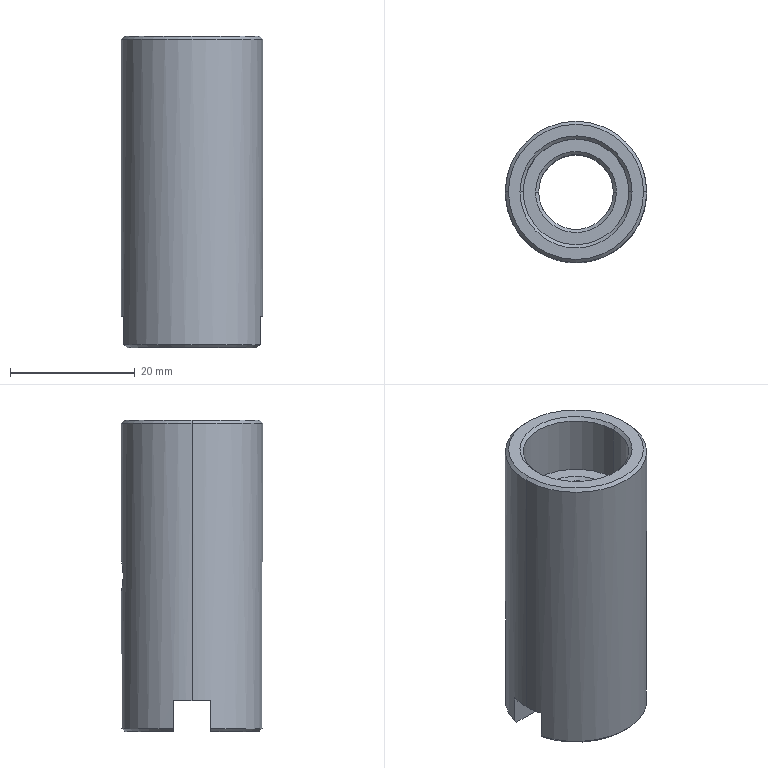Part | STEP file | 101000008215 | 1 solid | 28 faces | box 22.7 x 22.7 x 50 mm | volume 12976 mm3 | cone 10 | plane 10 | cylinder 8 | commonest cylinder face diameters 5 x2 12 x2 17 x2 22.7 x2
STEP:
#1=CARTESIAN_POINT('',(10.85,0.,50.));
#2=VERTEX_POINT('',#1);
#3=CARTESIAN_POINT('',(-10.85,0.,50.));
#4=VERTEX_POINT('',#3);
#5=CARTESIAN_POINT('',(0.,0.,50.));
#6=DIRECTION('',(0.,0.,-1.));
#7=AXIS2_PLACEMENT_3D('',#5,#6,$);
#8=CIRCLE('',#7,10.85);
#9=EDGE_CURVE('',#2,#4,#8,.F.);
#10=ORIENTED_EDGE('',*,*,#9,.F.);
#11=CARTESIAN_POINT('',(11.35,0.,49.5));
#12=VERTEX_POINT('',#11);
#13=CARTESIAN_POINT('',(353558.816,0.,-353497.966));
#14=DIRECTION('',(0.7071,0.,-0.7071));
#15=VECTOR('',#14,1.);
#16=LINE('',#13,#15);
#17=EDGE_CURVE('',#2,#12,#16,.T.);
#18=ORIENTED_EDGE('',*,*,#17,.T.);
#19=CARTESIAN_POINT('',(-11.35,0.,49.5));
#20=VERTEX_POINT('',#19);
#21=CARTESIAN_POINT('',(0.,0.,49.5));
#22=DIRECTION('',(0.,0.,-1.));
#23=AXIS2_PLACEMENT_3D('',#21,#22,$);
#24=CIRCLE('',#23,11.35);
#25=EDGE_CURVE('',#20,#12,#24,.T.);
#26=ORIENTED_EDGE('',*,*,#25,.F.);
#27=CARTESIAN_POINT('',(-353558.816,0.,-353497.966));
#28=DIRECTION('',(-0.7071,0.,-0.7071));
#29=VECTOR('',#28,1.);
#30=LINE('',#27,#29);
#31=EDGE_CURVE('',#4,#20,#30,.T.);
#32=ORIENTED_EDGE('',*,*,#31,.F.);
#33=EDGE_LOOP('',(#10,#18,#26,#32));
#34=FACE_OUTER_BOUND('',#33,.T.);
#35=CARTESIAN_POINT('',(0.,0.,50.));
#36=DIRECTION('',(0.,0.,-1.));
#37=DIRECTION('',(-1.,0.,0.));
#38=AXIS2_PLACEMENT_3D('',#35,#36,#37);
#39=CONICAL_SURFACE('',#38,10.85,0.7854);
#40=ADVANCED_FACE('',(#34),#39,.T.);
#41=CARTESIAN_POINT('',(0.,0.,50.));
#42=DIRECTION('',(0.,0.,1.));
#43=AXIS2_PLACEMENT_3D('',#41,#42,$);
#44=CIRCLE('',#43,10.85);
#45=EDGE_CURVE('',#4,#2,#44,.T.);
#46=ORIENTED_EDGE('',*,*,#45,.T.);
#47=ORIENTED_EDGE('',*,*,#9,.T.);
#48=EDGE_LOOP('',(#46,#47));
#49=FACE_OUTER_BOUND('',#48,.T.);
#50=CARTESIAN_POINT('',(9.,0.,50.));
#51=VERTEX_POINT('',#50);
#52=CARTESIAN_POINT('',(-9.,0.,50.));
#53=VERTEX_POINT('',#52);
#54=CARTESIAN_POINT('',(9.,0.,50.));
#55=CARTESIAN_POINT('',(9.,-0.8818,50.));
#56=CARTESIAN_POINT('',(8.892,-1.764,50.));
#57=CARTESIAN_POINT('',(8.676,-2.628,50.));
#58=CARTESIAN_POINT('',(8.037,-4.286,50.));
#59=CARTESIAN_POINT('',(7.016,-5.74,50.));
#60=CARTESIAN_POINT('',(6.419,-6.401,50.));
#61=CARTESIAN_POINT('',(5.075,-7.563,50.));
#62=CARTESIAN_POINT('',(3.49,-8.366,50.));
#63=CARTESIAN_POINT('',(2.652,-8.669,50.));
#64=CARTESIAN_POINT('',(0.9193,-9.061,50.));
#65=CARTESIAN_POINT('',(-0.8571,-9.025,50.));
#66=CARTESIAN_POINT('',(-1.739,-8.897,50.));
#67=CARTESIAN_POINT('',(-3.453,-8.428,50.));
#68=CARTESIAN_POINT('',(-5.003,-7.56,50.));
#69=CARTESIAN_POINT('',(-5.721,-7.032,50.));
#70=CARTESIAN_POINT('',(-7.012,-5.812,50.));
#71=CARTESIAN_POINT('',(-7.971,-4.317,50.));
#72=CARTESIAN_POINT('',(-8.357,-3.513,50.));
#73=CARTESIAN_POINT('',(-8.756,-2.324,50.));
#74=CARTESIAN_POINT('',(-8.945,-1.091,50.));
#75=CARTESIAN_POINT('',(-8.982,-0.7273,50.));
#76=CARTESIAN_POINT('',(-9.,-0.3637,50.));
#77=CARTESIAN_POINT('',(-9.,0.,50.));
#78=B_SPLINE_CURVE_WITH_KNOTS('',5,(#54,#55,#56,#57,#58,#59,#60,#61,#62,#63,#64,#65,#66,#67,#68,#69,#70,#71,#72,#73,#74,#75,#76,#77),.UNSPECIFIED.,.F.,.U.,(6,3,3,3,3,3,3,6),(0.,6.235,12.471,18.706,24.941,31.177,37.412,39.983),.UNSPECIFIED.);
#79=EDGE_CURVE('',#51,#53,#78,.T.);
#80=ORIENTED_EDGE('',*,*,#79,.T.);
#81=CARTESIAN_POINT('',(-9.,0.,50.));
#82=CARTESIAN_POINT('',(-9.,0.8818,50.));
#83=CARTESIAN_POINT('',(-8.892,1.764,50.));
#84=CARTESIAN_POINT('',(-8.676,2.628,50.));
#85=CARTESIAN_POINT('',(-8.037,4.286,50.));
#86=CARTESIAN_POINT('',(-7.016,5.74,50.));
#87=CARTESIAN_POINT('',(-6.419,6.401,50.));
#88=CARTESIAN_POINT('',(-5.075,7.563,50.));
#89=CARTESIAN_POINT('',(-3.49,8.366,50.));
#90=CARTESIAN_POINT('',(-2.652,8.669,50.));
#91=CARTESIAN_POINT('',(-0.9193,9.061,50.));
#92=CARTESIAN_POINT('',(0.8571,9.025,50.));
#93=CARTESIAN_POINT('',(1.739,8.897,50.));
#94=CARTESIAN_POINT('',(3.453,8.428,50.));
#95=CARTESIAN_POINT('',(5.003,7.56,50.));
#96=CARTESIAN_POINT('',(5.721,7.032,50.));
#97=CARTESIAN_POINT('',(7.012,5.812,50.));
#98=CARTESIAN_POINT('',(7.971,4.317,50.));
#99=CARTESIAN_POINT('',(8.357,3.513,50.));
#100=CARTESIAN_POINT('',(8.756,2.324,50.));
#101=CARTESIAN_POINT('',(8.945,1.091,50.));
#102=CARTESIAN_POINT('',(8.982,0.7273,50.));
#103=CARTESIAN_POINT('',(9.,0.3637,50.));
#104=CARTESIAN_POINT('',(9.,0.,50.));
#105=B_SPLINE_CURVE_WITH_KNOTS('',5,(#81,#82,#83,#84,#85,#86,#87,#88,#89,#90,#91,#92,#93,#94,#95,#96,#97,#98,#99,#100,#101,#102,#103,#104),.UNSPECIFIED.,.F.,.U.,(6,3,3,3,3,3,3,6),(0.,6.235,12.471,18.706,24.941,31.177,37.412,39.983),.UNSPECIFIED.);
#106=EDGE_CURVE('',#53,#51,#105,.T.);
#107=ORIENTED_EDGE('',*,*,#106,.T.);
#108=EDGE_LOOP('',(#80,#107));
#109=FACE_BOUND('',#108,.T.);
#110=CARTESIAN_POINT('',(0.,0.,50.));
#111=DIRECTION('',(0.,0.,1.));
#112=DIRECTION('',(1.,0.,0.));
#113=AXIS2_PLACEMENT_3D('',#110,#111,#112);
#114=PLANE('',#113);
#115=ADVANCED_FACE('',(#49,#109),#114,.T.);
#116=ORIENTED_EDGE('',*,*,#17,.F.);
#117=ORIENTED_EDGE('',*,*,#45,.F.);
#118=ORIENTED_EDGE('',*,*,#31,.T.);
#119=CARTESIAN_POINT('',(0.,0.,49.5));
#120=DIRECTION('',(0.,0.,-1.));
#121=AXIS2_PLACEMENT_3D('',#119,#120,$);
#122=CIRCLE('',#121,11.35);
#123=EDGE_CURVE('',#12,#20,#122,.T.);
#124=ORIENTED_EDGE('',*,*,#123,.F.);
#125=EDGE_LOOP('',(#116,#117,#118,#124));
#126=FACE_OUTER_BOUND('',#125,.T.);
#127=CARTESIAN_POINT('',(0.,0.,50.));
#128=DIRECTION('',(0.,0.,-1.));
#129=DIRECTION('',(1.,0.,0.));
#130=AXIS2_PLACEMENT_3D('',#127,#128,#129);
#131=CONICAL_SURFACE('',#130,10.85,0.7854);
#132=ADVANCED_FACE('',(#126),#131,.T.);
#133=ORIENTED_EDGE('',*,*,#25,.T.);
#134=CARTESIAN_POINT('',(11.35,0.,5.));
#135=VERTEX_POINT('',#134);
#136=CARTESIAN_POINT('',(11.35,0.,50.));
#137=DIRECTION('',(0.,0.,-1.));
#138=VECTOR('',#137,1.);
#139=LINE('',#136,#138);
#140=EDGE_CURVE('',#12,#135,#139,.T.);
#141=ORIENTED_EDGE('',*,*,#140,.T.);
#142=CARTESIAN_POINT('',(10.946,3.,5.));
#143=VERTEX_POINT('',#142);
#144=CARTESIAN_POINT('',(0.,0.,5.));
#145=DIRECTION('',(0.,0.,-1.));
#146=AXIS2_PLACEMENT_3D('',#144,#145,$);
#147=CIRCLE('',#146,11.35);
#148=EDGE_CURVE('',#135,#143,#147,.F.);
#149=ORIENTED_EDGE('',*,*,#148,.T.);
#150=CARTESIAN_POINT('',(10.946,3.,0.5));
#151=VERTEX_POINT('',#150);
#152=CARTESIAN_POINT('',(10.946,3.,50.));
#153=DIRECTION('',(0.,0.,-1.));
#154=VECTOR('',#153,1.);
#155=LINE('',#152,#154);
#156=EDGE_CURVE('',#143,#151,#155,.T.);
#157=ORIENTED_EDGE('',*,*,#156,.T.);
#158=CARTESIAN_POINT('',(-10.946,3.,0.5));
#159=VERTEX_POINT('',#158);
#160=CARTESIAN_POINT('',(0.,0.,0.5));
#161=DIRECTION('',(0.,0.,-1.));
#162=AXIS2_PLACEMENT_3D('',#160,#161,$);
#163=CIRCLE('',#162,11.35);
#164=EDGE_CURVE('',#151,#159,#163,.F.);
#165=ORIENTED_EDGE('',*,*,#164,.T.);
#166=CARTESIAN_POINT('',(-10.946,3.,5.));
#167=VERTEX_POINT('',#166);
#168=CARTESIAN_POINT('',(-10.946,3.,50.));
#169=DIRECTION('',(0.,0.,-1.));
#170=VECTOR('',#169,1.);
#171=LINE('',#168,#170);
#172=EDGE_CURVE('',#159,#167,#171,.F.);
#173=ORIENTED_EDGE('',*,*,#172,.T.);
#174=CARTESIAN_POINT('',(-11.35,0.,5.));
#175=VERTEX_POINT('',#174);
#176=CARTESIAN_POINT('',(0.,0.,5.));
#177=DIRECTION('',(0.,0.,-1.));
#178=AXIS2_PLACEMENT_3D('',#176,#177,$);
#179=CIRCLE('',#178,11.35);
#180=EDGE_CURVE('',#167,#175,#179,.F.);
#181=ORIENTED_EDGE('',*,*,#180,.T.);
#182=CARTESIAN_POINT('',(-11.35,0.,50.));
#183=DIRECTION('',(0.,0.,-1.));
#184=VECTOR('',#183,1.);
#185=LINE('',#182,#184);
#186=EDGE_CURVE('',#20,#175,#185,.T.);
#187=ORIENTED_EDGE('',*,*,#186,.F.);
#188=EDGE_LOOP('',(#133,#141,#149,#157,#165,#173,#181,#187));
#189=FACE_OUTER_BOUND('',#188,.T.);
#190=CARTESIAN_POINT('',(0.,11.35,27.5));
#191=VERTEX_POINT('',#190);
#192=CARTESIAN_POINT('',(0.,11.35,22.5));
#193=VERTEX_POINT('',#192);
#194=CARTESIAN_POINT('',(0.,11.35,27.5));
#195=CARTESIAN_POINT('',(-0.2311,11.35,27.5));
#196=CARTESIAN_POINT('',(-0.4593,11.344,27.474));
#197=CARTESIAN_POINT('',(-0.687,11.332,27.42));
#198=CARTESIAN_POINT('',(-1.051,11.305,27.289));
#199=CARTESIAN_POINT('',(-1.38,11.267,27.093));
#200=CARTESIAN_POINT('',(-1.506,11.251,27.004));
#201=CARTESIAN_POINT('',(-1.922,11.191,26.66));
#202=CARTESIAN_POINT('',(-2.236,11.13,26.214));
#203=CARTESIAN_POINT('',(-2.398,11.094,25.852));
#204=CARTESIAN_POINT('',(-2.52,11.067,25.32));
#205=CARTESIAN_POINT('',(-2.497,11.072,24.78));
#206=CARTESIAN_POINT('',(-2.479,11.076,24.626));
#207=CARTESIAN_POINT('',(-2.404,11.093,24.249));
#208=CARTESIAN_POINT('',(-2.259,11.124,23.893));
#209=CARTESIAN_POINT('',(-2.148,11.146,23.689));
#210=CARTESIAN_POINT('',(-1.878,11.196,23.31));
#211=CARTESIAN_POINT('',(-1.531,11.248,23.003));
#212=CARTESIAN_POINT('',(-1.339,11.273,22.87));
#213=CARTESIAN_POINT('',(-0.9666,11.313,22.671));
#214=CARTESIAN_POINT('',(-0.5631,11.338,22.553));
#215=CARTESIAN_POINT('',(-0.3767,11.346,22.518));
#216=CARTESIAN_POINT('',(-0.1878,11.35,22.5));
#217=CARTESIAN_POINT('',(0.,11.35,22.5));
#218=B_SPLINE_CURVE_WITH_KNOTS('',5,(#194,#195,#196,#197,#198,#199,#200,#201,#202,#203,#204,#205,#206,#207,#208,#209,#210,#211,#212,#213,#214,#215,#216,#217),.UNSPECIFIED.,.F.,.U.,(6,3,3,3,3,3,3,6),(0.,1.627,2.724,5.45,6.533,8.168,9.815,11.146),.UNSPECIFIED.);
#219=EDGE_CURVE('',#191,#193,#218,.T.);
#220=ORIENTED_EDGE('',*,*,#219,.T.);
#221=CARTESIAN_POINT('',(0.,11.35,22.5));
#222=CARTESIAN_POINT('',(0.2297,11.35,22.5));
#223=CARTESIAN_POINT('',(0.4594,11.344,22.527));
#224=CARTESIAN_POINT('',(0.6875,11.332,22.58));
#225=CARTESIAN_POINT('',(1.051,11.305,22.711));
#226=CARTESIAN_POINT('',(1.381,11.267,22.908));
#227=CARTESIAN_POINT('',(1.508,11.25,22.997));
#228=CARTESIAN_POINT('',(1.745,11.216,23.193));
#229=CARTESIAN_POINT('',(1.95,11.182,23.425));
#230=CARTESIAN_POINT('',(2.044,11.165,23.549));
#231=CARTESIAN_POINT('',(2.252,11.125,23.871));
#232=CARTESIAN_POINT('',(2.395,11.095,24.229));
#233=CARTESIAN_POINT('',(2.455,11.081,24.455));
#234=CARTESIAN_POINT('',(2.513,11.068,24.835));
#235=CARTESIAN_POINT('',(2.498,11.072,25.218));
#236=CARTESIAN_POINT('',(2.479,11.076,25.371));
#237=CARTESIAN_POINT('',(2.42,11.089,25.673));
#238=CARTESIAN_POINT('',(2.315,11.112,25.962));
#239=CARTESIAN_POINT('',(2.252,11.125,26.101));
#240=CARTESIAN_POINT('',(2.104,11.154,26.373));
#241=CARTESIAN_POINT('',(1.915,11.188,26.618));
#242=CARTESIAN_POINT('',(1.811,11.205,26.734));
#243=CARTESIAN_POINT('',(1.451,11.261,27.076));
#244=CARTESIAN_POINT('',(1.014,11.311,27.323));
#245=CARTESIAN_POINT('',(0.6857,11.337,27.441));
#246=CARTESIAN_POINT('',(0.3439,11.35,27.5));
#247=CARTESIAN_POINT('',(0.,11.35,27.5));
#248=B_SPLINE_CURVE_WITH_KNOTS('',5,(#221,#222,#223,#224,#225,#226,#227,#228,#229,#230,#231,#232,#233,#234,#235,#236,#237,#238,#239,#240,#241,#242,#243,#244,#245,#246,#247),.UNSPECIFIED.,.F.,.U.,(6,3,3,3,3,3,3,3,6),(0.,1.629,2.725,3.823,5.451,6.53,7.624,8.727,11.154),.UNSPECIFIED.);
#249=EDGE_CURVE('',#193,#191,#248,.T.);
#250=ORIENTED_EDGE('',*,*,#249,.T.);
#251=EDGE_LOOP('',(#220,#250));
#252=FACE_BOUND('',#251,.T.);
#253=CARTESIAN_POINT('',(0.,0.,50.));
#254=DIRECTION('',(0.,0.,-1.));
#255=DIRECTION('',(-1.,0.,0.));
#256=AXIS2_PLACEMENT_3D('',#253,#254,#255);
#257=CYLINDRICAL_SURFACE('',#256,11.35);
#258=ADVANCED_FACE('',(#189,#252),#257,.T.);
#259=CARTESIAN_POINT('',(-8.5,0.,49.5));
#260=VERTEX_POINT('',#259);
#261=CARTESIAN_POINT('',(8.5,0.,49.5));
#262=VERTEX_POINT('',#261);
#263=CARTESIAN_POINT('',(0.,0.,49.5));
#264=DIRECTION('',(0.,0.,1.));
#265=AXIS2_PLACEMENT_3D('',#263,#264,$);
#266=CIRCLE('',#265,8.5);
#267=EDGE_CURVE('',#260,#262,#266,.T.);
#268=ORIENTED_EDGE('',*,*,#267,.F.);
#269=CARTESIAN_POINT('',(-353557.641,0.,353598.641));
#270=DIRECTION('',(-0.7071,0.,0.7071));
#271=VECTOR('',#270,1.);
#272=LINE('',#269,#271);
#273=EDGE_CURVE('',#260,#53,#272,.T.);
#274=ORIENTED_EDGE('',*,*,#273,.T.);
#275=ORIENTED_EDGE('',*,*,#79,.F.);
#276=CARTESIAN_POINT('',(353557.641,0.,353598.641));
#277=DIRECTION('',(0.7071,0.,0.7071));
#278=VECTOR('',#277,1.);
#279=LINE('',#276,#278);
#280=EDGE_CURVE('',#262,#51,#279,.T.);
#281=ORIENTED_EDGE('',*,*,#280,.F.);
#282=EDGE_LOOP('',(#268,#274,#275,#281));
#283=FACE_OUTER_BOUND('',#282,.T.);
#284=CARTESIAN_POINT('',(0.,0.,49.5));
#285=DIRECTION('',(0.,0.,1.));
#286=DIRECTION('',(-1.,0.,0.));
#287=AXIS2_PLACEMENT_3D('',#284,#285,#286);
#288=CONICAL_SURFACE('',#287,8.5,0.7854);
#289=ADVANCED_FACE('',(#283),#288,.F.);
#290=ORIENTED_EDGE('',*,*,#273,.F.);
#291=CARTESIAN_POINT('',(0.,0.,49.5));
#292=DIRECTION('',(0.,0.,1.));
#293=AXIS2_PLACEMENT_3D('',#291,#292,$);
#294=CIRCLE('',#293,8.5);
#295=EDGE_CURVE('',#262,#260,#294,.T.);
#296=ORIENTED_EDGE('',*,*,#295,.F.);
#297=ORIENTED_EDGE('',*,*,#280,.T.);
#298=ORIENTED_EDGE('',*,*,#106,.F.);
#299=EDGE_LOOP('',(#290,#296,#297,#298));
#300=FACE_OUTER_BOUND('',#299,.T.);
#301=CARTESIAN_POINT('',(0.,0.,49.5));
#302=DIRECTION('',(0.,0.,1.));
#303=DIRECTION('',(1.,0.,0.));
#304=AXIS2_PLACEMENT_3D('',#301,#302,#303);
#305=CONICAL_SURFACE('',#304,8.5,0.7854);
#306=ADVANCED_FACE('',(#300),#305,.F.);
#307=ORIENTED_EDGE('',*,*,#140,.F.);
#308=ORIENTED_EDGE('',*,*,#123,.T.);
#309=ORIENTED_EDGE('',*,*,#186,.T.);
#310=CARTESIAN_POINT('',(-10.946,-3.,5.));
#311=VERTEX_POINT('',#310);
#312=CARTESIAN_POINT('',(0.,0.,5.));
#313=DIRECTION('',(0.,0.,-1.));
#314=AXIS2_PLACEMENT_3D('',#312,#313,$);
#315=CIRCLE('',#314,11.35);
#316=EDGE_CURVE('',#175,#311,#315,.F.);
#317=ORIENTED_EDGE('',*,*,#316,.T.);
#318=CARTESIAN_POINT('',(-10.946,-3.,0.5));
#319=VERTEX_POINT('',#318);
#320=CARTESIAN_POINT('',(-10.946,-3.,50.));
#321=DIRECTION('',(0.,0.,-1.));
#322=VECTOR('',#321,1.);
#323=LINE('',#320,#322);
#324=EDGE_CURVE('',#311,#319,#323,.T.);
#325=ORIENTED_EDGE('',*,*,#324,.T.);
#326=CARTESIAN_POINT('',(10.946,-3.,0.5));
#327=VERTEX_POINT('',#326);
#328=CARTESIAN_POINT('',(0.,0.,0.5));
#329=DIRECTION('',(0.,0.,-1.));
#330=AXIS2_PLACEMENT_3D('',#328,#329,$);
#331=CIRCLE('',#330,11.35);
#332=EDGE_CURVE('',#319,#327,#331,.F.);
#333=ORIENTED_EDGE('',*,*,#332,.T.);
#334=CARTESIAN_POINT('',(10.946,-3.,5.));
#335=VERTEX_POINT('',#334);
#336=CARTESIAN_POINT('',(10.946,-3.,50.));
#337=DIRECTION('',(0.,0.,-1.));
#338=VECTOR('',#337,1.);
#339=LINE('',#336,#338);
#340=EDGE_CURVE('',#327,#335,#339,.F.);
#341=ORIENTED_EDGE('',*,*,#340,.T.);
#342=CARTESIAN_POINT('',(0.,0.,5.));
#343=DIRECTION('',(0.,0.,-1.));
#344=AXIS2_PLACEMENT_3D('',#342,#343,$);
#345=CIRCLE('',#344,11.35);
#346=EDGE_CURVE('',#335,#135,#345,.F.);
#347=ORIENTED_EDGE('',*,*,#346,.T.);
#348=EDGE_LOOP('',(#307,#308,#309,#317,#325,#333,#341,#347));
#349=FACE_OUTER_BOUND('',#348,.T.);
#350=CARTESIAN_POINT('',(0.,0.,50.));
#351=DIRECTION('',(0.,0.,-1.));
#352=DIRECTION('',(1.,0.,0.));
#353=AXIS2_PLACEMENT_3D('',#350,#351,#352);
#354=CYLINDRICAL_SURFACE('',#353,11.35);
#355=ADVANCED_FACE('',(#349),#354,.T.);
#356=CARTESIAN_POINT('',(5.196,-3.,5.));
#357=VERTEX_POINT('',#356);
#358=CARTESIAN_POINT('',(6.,0.,5.));
#359=VERTEX_POINT('',#358);
#360=CARTESIAN_POINT('',(0.00000002,-0.000000005,5.));
#361=DIRECTION('',(0.,0.,1.));
#362=AXIS2_PLACEMENT_3D('',#360,#361,$);
#363=CIRCLE('',#362,6.);
#364=EDGE_CURVE('',#357,#359,#363,.T.);
#365=ORIENTED_EDGE('',*,*,#364,.T.);
#366=CARTESIAN_POINT('',(5.196,3.,5.));
#367=VERTEX_POINT('',#366);
#368=CARTESIAN_POINT('',(0.00000002,0.000000005,5.));
#369=DIRECTION('',(0.,0.,1.));
#370=AXIS2_PLACEMENT_3D('',#368,#369,$);
#371=CIRCLE('',#370,6.);
#372=EDGE_CURVE('',#359,#367,#371,.T.);
#373=ORIENTED_EDGE('',*,*,#372,.T.);
#374=CARTESIAN_POINT('',(8.071,3.,5.));
#375=DIRECTION('',(1.,0.,0.));
#376=VECTOR('',#375,1.);
#377=LINE('',#374,#376);
#378=EDGE_CURVE('',#367,#143,#377,.T.);
#379=ORIENTED_EDGE('',*,*,#378,.T.);
#380=ORIENTED_EDGE('',*,*,#148,.F.);
#381=ORIENTED_EDGE('',*,*,#346,.F.);
#382=CARTESIAN_POINT('',(8.071,-3.,5.));
#383=DIRECTION('',(1.,0.,0.));
#384=VECTOR('',#383,1.);
#385=LINE('',#382,#384);
#386=EDGE_CURVE('',#357,#335,#385,.T.);
#387=ORIENTED_EDGE('',*,*,#386,.F.);
#388=EDGE_LOOP('',(#365,#373,#379,#380,#381,#387));
#389=FACE_OUTER_BOUND('',#388,.T.);
#390=CARTESIAN_POINT('',(-11.35,3.,5.));
#391=DIRECTION('',(0.,0.,1.));
#392=DIRECTION('',(1.,0.,0.));
#393=AXIS2_PLACEMENT_3D('',#390,#391,#392);
#394=PLANE('',#393);
#395=ADVANCED_FACE('',(#389),#394,.F.);
#396=CARTESIAN_POINT('',(5.766,3.,0.));
#397=VERTEX_POINT('',#396);
#398=CARTESIAN_POINT('',(10.427,3.,0.));
#399=VERTEX_POINT('',#398);
#400=CARTESIAN_POINT('',(8.097,3.,0.));
#401=DIRECTION('',(1.,0.,0.));
#402=VECTOR('',#401,1.);
#403=LINE('',#400,#402);
#404=EDGE_CURVE('',#397,#399,#403,.T.);
#405=ORIENTED_EDGE('',*,*,#404,.T.);
#406=CARTESIAN_POINT('',(10.427,3.,0.));
#407=CARTESIAN_POINT('',(10.531,3.,0.09991));
#408=CARTESIAN_POINT('',(10.635,3.,0.1999));
#409=CARTESIAN_POINT('',(10.739,3.,0.2999));
#410=CARTESIAN_POINT('',(10.843,3.,0.3999));
#411=CARTESIAN_POINT('',(10.946,3.,0.5));
#412=B_SPLINE_CURVE_WITH_KNOTS('',5,(#406,#407,#408,#409,#410,#411),.UNSPECIFIED.,.F.,.U.,(6,6),(0.,1.02),.UNSPECIFIED.);
#413=EDGE_CURVE('',#399,#151,#412,.T.);
#414=ORIENTED_EDGE('',*,*,#413,.T.);
#415=ORIENTED_EDGE('',*,*,#156,.F.);
#416=ORIENTED_EDGE('',*,*,#378,.F.);
#417=CARTESIAN_POINT('',(5.196,3.,0.5));
#418=VERTEX_POINT('',#417);
#419=CARTESIAN_POINT('',(5.196,3.,2.75));
#420=DIRECTION('',(0.,0.,-1.));
#421=VECTOR('',#420,1.);
#422=LINE('',#419,#421);
#423=EDGE_CURVE('',#367,#418,#422,.T.);
#424=ORIENTED_EDGE('',*,*,#423,.T.);
#425=CARTESIAN_POINT('',(5.196,3.,0.5));
#426=CARTESIAN_POINT('',(5.311,3.,0.4007));
#427=CARTESIAN_POINT('',(5.425,3.,0.301));
#428=CARTESIAN_POINT('',(5.539,3.,0.201));
#429=CARTESIAN_POINT('',(5.653,3.,0.1006));
#430=CARTESIAN_POINT('',(5.766,3.,0.));
#431=B_SPLINE_CURVE_WITH_KNOTS('',5,(#425,#426,#427,#428,#429,#430),.UNSPECIFIED.,.F.,.U.,(6,6),(0.,1.072),.UNSPECIFIED.);
#432=EDGE_CURVE('',#418,#397,#431,.T.);
#433=ORIENTED_EDGE('',*,*,#432,.T.);
#434=EDGE_LOOP('',(#405,#414,#415,#416,#424,#433));
#435=FACE_OUTER_BOUND('',#434,.T.);
#436=CARTESIAN_POINT('',(-11.35,3.,5.));
#437=DIRECTION('',(0.,1.,0.));
#438=DIRECTION('',(0.,0.,1.));
#439=AXIS2_PLACEMENT_3D('',#436,#437,#438);
#440=PLANE('',#439);
#441=ADVANCED_FACE('',(#435),#440,.F.);
#442=ORIENTED_EDGE('',*,*,#413,.F.);
#443=CARTESIAN_POINT('',(-10.427,3.,0.));
#444=VERTEX_POINT('',#443);
#445=CARTESIAN_POINT('',(0.,0.,0.));
#446=DIRECTION('',(0.,0.,1.));
#447=AXIS2_PLACEMENT_3D('',#445,#446,$);
#448=CIRCLE('',#447,10.85);
#449=EDGE_CURVE('',#444,#399,#448,.F.);
#450=ORIENTED_EDGE('',*,*,#449,.F.);
#451=CARTESIAN_POINT('',(-10.946,3.,0.5));
#452=CARTESIAN_POINT('',(-10.769,3.,0.3286));
#453=CARTESIAN_POINT('',(-10.595,3.,0.1619));
#454=CARTESIAN_POINT('',(-10.427,3.,0.));
#455=B_SPLINE_CURVE_WITH_KNOTS('',3,(#451,#452,#453,#454),.UNSPECIFIED.,.F.,.U.,(4,4),(0.,1.619),.UNSPECIFIED.);
#456=EDGE_CURVE('',#159,#444,#455,.T.);
#457=ORIENTED_EDGE('',*,*,#456,.F.);
#458=ORIENTED_EDGE('',*,*,#164,.F.);
#459=EDGE_LOOP('',(#442,#450,#457,#458));
#460=FACE_OUTER_BOUND('',#459,.T.);
#461=CARTESIAN_POINT('',(0.,0.,0.5));
#462=DIRECTION('',(0.,0.,1.));
#463=DIRECTION('',(1.,0.,0.));
#464=AXIS2_PLACEMENT_3D('',#461,#462,#463);
#465=CONICAL_SURFACE('',#464,11.35,0.7854);
#466=ADVANCED_FACE('',(#460),#465,.T.);
#467=ORIENTED_EDGE('',*,*,#172,.F.);
#468=ORIENTED_EDGE('',*,*,#456,.T.);
#469=CARTESIAN_POINT('',(-5.766,3.,0.));
#470=VERTEX_POINT('',#469);
#471=CARTESIAN_POINT('',(-8.097,3.,0.));
#472=DIRECTION('',(1.,0.,0.));
#473=VECTOR('',#472,1.);
#474=LINE('',#471,#473);
#475=EDGE_CURVE('',#444,#470,#474,.T.);
#476=ORIENTED_EDGE('',*,*,#475,.T.);
#477=CARTESIAN_POINT('',(-5.196,3.,0.5));
#478=VERTEX_POINT('',#477);
#479=CARTESIAN_POINT('',(-5.766,3.,0.));
#480=CARTESIAN_POINT('',(-5.653,3.,0.1006));
#481=CARTESIAN_POINT('',(-5.539,3.,0.201));
#482=CARTESIAN_POINT('',(-5.425,3.,0.301));
#483=CARTESIAN_POINT('',(-5.311,3.,0.4007));
#484=CARTESIAN_POINT('',(-5.196,3.,0.5));
#485=B_SPLINE_CURVE_WITH_KNOTS('',5,(#479,#480,#481,#482,#483,#484),.UNSPECIFIED.,.F.,.U.,(6,6),(0.,1.072),.UNSPECIFIED.);
#486=EDGE_CURVE('',#470,#478,#485,.T.);
#487=ORIENTED_EDGE('',*,*,#486,.T.);
#488=CARTESIAN_POINT('',(-5.196,3.,5.));
#489=VERTEX_POINT('',#488);
#490=CARTESIAN_POINT('',(-5.196,3.,2.75));
#491=DIRECTION('',(0.,0.,1.));
#492=VECTOR('',#491,1.);
#493=LINE('',#490,#492);
#494=EDGE_CURVE('',#478,#489,#493,.T.);
#495=ORIENTED_EDGE('',*,*,#494,.T.);
#496=CARTESIAN_POINT('',(-8.071,3.,5.));
#497=DIRECTION('',(1.,0.,0.));
#498=VECTOR('',#497,1.);
#499=LINE('',#496,#498);
#500=EDGE_CURVE('',#167,#489,#499,.T.);
#501=ORIENTED_EDGE('',*,*,#500,.F.);
#502=EDGE_LOOP('',(#467,#468,#476,#487,#495,#501));
#503=FACE_OUTER_BOUND('',#502,.T.);
#504=CARTESIAN_POINT('',(-11.35,3.,5.));
#505=DIRECTION('',(0.,1.,0.));
#506=DIRECTION('',(0.,0.,1.));
#507=AXIS2_PLACEMENT_3D('',#504,#505,#506);
#508=PLANE('',#507);
#509=ADVANCED_FACE('',(#503),#508,.F.);
#510=CARTESIAN_POINT('',(-6.,0.,5.));
#511=VERTEX_POINT('',#510);
#512=CARTESIAN_POINT('',(-0.000000021,0.000000005,5.));
#513=DIRECTION('',(0.,0.,1.));
#514=AXIS2_PLACEMENT_3D('',#512,#513,$);
#515=CIRCLE('',#514,6.);
#516=EDGE_CURVE('',#489,#511,#515,.T.);
#517=ORIENTED_EDGE('',*,*,#516,.T.);
#518=CARTESIAN_POINT('',(-5.196,-3.,5.));
#519=VERTEX_POINT('',#518);
#520=CARTESIAN_POINT('',(-0.000000021,-0.000000005,5.));
#521=DIRECTION('',(0.,0.,1.));
#522=AXIS2_PLACEMENT_3D('',#520,#521,$);
#523=CIRCLE('',#522,6.);
#524=EDGE_CURVE('',#511,#519,#523,.T.);
#525=ORIENTED_EDGE('',*,*,#524,.T.);
#526=CARTESIAN_POINT('',(-8.071,-3.,5.));
#527=DIRECTION('',(1.,0.,0.));
#528=VECTOR('',#527,1.);
#529=LINE('',#526,#528);
#530=EDGE_CURVE('',#311,#519,#529,.T.);
#531=ORIENTED_EDGE('',*,*,#530,.F.);
#532=ORIENTED_EDGE('',*,*,#316,.F.);
#533=ORIENTED_EDGE('',*,*,#180,.F.);
#534=ORIENTED_EDGE('',*,*,#500,.T.);
#535=EDGE_LOOP('',(#517,#525,#531,#532,#533,#534));
#536=FACE_OUTER_BOUND('',#535,.T.);
#537=CARTESIAN_POINT('',(-11.35,3.,5.));
#538=DIRECTION('',(0.,0.,1.));
#539=DIRECTION('',(1.,0.,0.));
#540=AXIS2_PLACEMENT_3D('',#537,#538,#539);
#541=PLANE('',#540);
#542=ADVANCED_FACE('',(#536),#541,.F.);
#543=CARTESIAN_POINT('',(0.,6.,27.5));
#544=VERTEX_POINT('',#543);
#545=CARTESIAN_POINT('',(0.,6.,22.5));
#546=VERTEX_POINT('',#545);
#547=CARTESIAN_POINT('',(0.,6.,27.5));
#548=CARTESIAN_POINT('',(-0.3045,6.,27.5));
#549=CARTESIAN_POINT('',(-0.6041,5.981,27.454));
#550=CARTESIAN_POINT('',(-0.8951,5.943,27.363));
#551=CARTESIAN_POINT('',(-1.308,5.864,27.162));
#552=CARTESIAN_POINT('',(-1.663,5.767,26.877));
#553=CARTESIAN_POINT('',(-1.769,5.735,26.777));
#554=CARTESIAN_POINT('',(-1.976,5.667,26.55));
#555=CARTESIAN_POINT('',(-2.147,5.604,26.294));
#556=CARTESIAN_POINT('',(-2.222,5.574,26.16));
#557=CARTESIAN_POINT('',(-2.349,5.522,25.888));
#558=CARTESIAN_POINT('',(-2.434,5.484,25.599));
#559=CARTESIAN_POINT('',(-2.465,5.47,25.456));
#560=CARTESIAN_POINT('',(-2.506,5.452,25.162));
#561=CARTESIAN_POINT('',(-2.503,5.453,24.864));
#562=CARTESIAN_POINT('',(-2.49,5.459,24.713));
#563=CARTESIAN_POINT('',(-2.442,5.481,24.417));
#564=CARTESIAN_POINT('',(-2.352,5.52,24.133));
#565=CARTESIAN_POINT('',(-2.296,5.544,23.994));
#566=CARTESIAN_POINT('',(-2.161,5.599,23.721));
#567=CARTESIAN_POINT('',(-1.988,5.662,23.472));
#568=CARTESIAN_POINT('',(-1.89,5.696,23.353));
#569=CARTESIAN_POINT('',(-1.628,5.78,23.079));
#570=CARTESIAN_POINT('',(-1.318,5.858,22.858));
#571=CARTESIAN_POINT('',(-1.115,5.902,22.745));
#572=CARTESIAN_POINT('',(-0.7752,5.956,22.605));
#573=CARTESIAN_POINT('',(-0.415,5.988,22.529));
#574=CARTESIAN_POINT('',(-0.2773,5.996,22.51));
#575=CARTESIAN_POINT('',(-0.1387,6.,22.5));
#576=CARTESIAN_POINT('',(0.,6.,22.5));
#577=B_SPLINE_CURVE_WITH_KNOTS('',5,(#547,#548,#549,#550,#551,#552,#553,#554,#555,#556,#557,#558,#559,#560,#561,#562,#563,#564,#565,#566,#567,#568,#569,#570,#571,#572,#573,#574,#575,#576),.UNSPECIFIED.,.F.,.U.,(6,3,3,3,3,3,3,3,3,6),(0.,2.145,3.277,4.365,5.422,6.468,7.54,8.653,10.281,11.264),.UNSPECIFIED.);
#578=EDGE_CURVE('',#544,#546,#577,.T.);
#579=ORIENTED_EDGE('',*,*,#578,.T.);
#580=CARTESIAN_POINT('',(0.,11.5,22.5));
#581=DIRECTION('',(0.,1.,0.));
#582=VECTOR('',#581,1.);
#583=LINE('',#580,#582);
#584=EDGE_CURVE('',#546,#193,#583,.T.);
#585=ORIENTED_EDGE('',*,*,#584,.T.);
#586=ORIENTED_EDGE('',*,*,#219,.F.);
#587=CARTESIAN_POINT('',(0.,11.5,27.5));
#588=DIRECTION('',(0.,1.,0.));
#589=VECTOR('',#588,1.);
#590=LINE('',#587,#589);
#591=EDGE_CURVE('',#544,#191,#590,.T.);
#592=ORIENTED_EDGE('',*,*,#591,.F.);
#593=EDGE_LOOP('',(#579,#585,#586,#592));
#594=FACE_OUTER_BOUND('',#593,.T.);
#595=CARTESIAN_POINT('',(0.,11.5,25.));
#596=DIRECTION('',(0.,1.,0.));
#597=DIRECTION('',(0.,0.,-1.));
#598=AXIS2_PLACEMENT_3D('',#595,#596,#597);
#599=CYLINDRICAL_SURFACE('',#598,2.5);
#600=ADVANCED_FACE('',(#594),#599,.F.);
#601=ORIENTED_EDGE('',*,*,#584,.F.);
#602=CARTESIAN_POINT('',(0.,6.,22.5));
#603=CARTESIAN_POINT('',(0.3012,6.,22.5));
#604=CARTESIAN_POINT('',(0.6054,5.98,22.545));
#605=CARTESIAN_POINT('',(0.8939,5.943,22.636));
#606=CARTESIAN_POINT('',(1.308,5.864,22.838));
#607=CARTESIAN_POINT('',(1.661,5.768,23.121));
#608=CARTESIAN_POINT('',(1.765,5.736,23.22));
#609=CARTESIAN_POINT('',(1.973,5.669,23.445));
#610=CARTESIAN_POINT('',(2.144,5.605,23.701));
#611=CARTESIAN_POINT('',(2.22,5.575,23.835));
#612=CARTESIAN_POINT('',(2.378,5.51,24.172));
#613=CARTESIAN_POINT('',(2.471,5.468,24.535));
#614=CARTESIAN_POINT('',(2.503,5.452,24.759));
#615=CARTESIAN_POINT('',(2.521,5.445,25.369));
#616=CARTESIAN_POINT('',(2.356,5.521,25.959));
#617=CARTESIAN_POINT('',(2.182,5.596,26.304));
#618=CARTESIAN_POINT('',(1.73,5.763,26.898));
#619=CARTESIAN_POINT('',(1.091,5.914,27.294));
#620=CARTESIAN_POINT('',(0.7403,5.971,27.43));
#621=CARTESIAN_POINT('',(0.3732,6.,27.5));
#622=CARTESIAN_POINT('',(0.,6.,27.5));
#623=B_SPLINE_CURVE_WITH_KNOTS('',5,(#602,#603,#604,#605,#606,#607,#608,#609,#610,#611,#612,#613,#614,#615,#616,#617,#618,#619,#620,#621,#622),.UNSPECIFIED.,.F.,.U.,(6,3,3,3,3,3,6),(0.,2.138,3.265,4.357,5.931,8.64,11.265),.UNSPECIFIED.);
#624=EDGE_CURVE('',#546,#544,#623,.T.);
#625=ORIENTED_EDGE('',*,*,#624,.T.);
#626=ORIENTED_EDGE('',*,*,#591,.T.);
#627=ORIENTED_EDGE('',*,*,#249,.F.);
#628=EDGE_LOOP('',(#601,#625,#626,#627));
#629=FACE_OUTER_BOUND('',#628,.T.);
#630=CARTESIAN_POINT('',(0.,11.5,25.));
#631=DIRECTION('',(0.,1.,0.));
#632=DIRECTION('',(0.,0.,1.));
#633=AXIS2_PLACEMENT_3D('',#630,#631,#632);
#634=CYLINDRICAL_SURFACE('',#633,2.5);
#635=ADVANCED_FACE('',(#629),#634,.F.);
#636=CARTESIAN_POINT('',(-8.5,0.,40.));
#637=VERTEX_POINT('',#636);
#638=CARTESIAN_POINT('',(8.5,0.,40.));
#639=VERTEX_POINT('',#638);
#640=CARTESIAN_POINT('',(0.,0.,40.));
#641=DIRECTION('',(0.,0.,1.));
#642=AXIS2_PLACEMENT_3D('',#640,#641,$);
#643=CIRCLE('',#642,8.5);
#644=EDGE_CURVE('',#637,#639,#643,.T.);
#645=ORIENTED_EDGE('',*,*,#644,.F.);
#646=CARTESIAN_POINT('',(-8.5,0.,40.));
#647=DIRECTION('',(0.,0.,1.));
#648=VECTOR('',#647,1.);
#649=LINE('',#646,#648);
#650=EDGE_CURVE('',#637,#260,#649,.T.);
#651=ORIENTED_EDGE('',*,*,#650,.T.);
#652=ORIENTED_EDGE('',*,*,#267,.T.);
#653=CARTESIAN_POINT('',(8.5,0.,40.));
#654=DIRECTION('',(0.,0.,1.));
#655=VECTOR('',#654,1.);
#656=LINE('',#653,#655);
#657=EDGE_CURVE('',#639,#262,#656,.T.);
#658=ORIENTED_EDGE('',*,*,#657,.F.);
#659=EDGE_LOOP('',(#645,#651,#652,#658));
#660=FACE_OUTER_BOUND('',#659,.T.);
#661=CARTESIAN_POINT('',(0.,0.,40.));
#662=DIRECTION('',(0.,0.,1.));
#663=DIRECTION('',(-1.,0.,0.));
#664=AXIS2_PLACEMENT_3D('',#661,#662,#663);
#665=CYLINDRICAL_SURFACE('',#664,8.5);
#666=ADVANCED_FACE('',(#660),#665,.F.);
#667=ORIENTED_EDGE('',*,*,#650,.F.);
#668=CARTESIAN_POINT('',(0.,0.,40.));
#669=DIRECTION('',(0.,0.,1.));
#670=AXIS2_PLACEMENT_3D('',#668,#669,$);
#671=CIRCLE('',#670,8.5);
#672=EDGE_CURVE('',#639,#637,#671,.T.);
#673=ORIENTED_EDGE('',*,*,#672,.F.);
#674=ORIENTED_EDGE('',*,*,#657,.T.);
#675=ORIENTED_EDGE('',*,*,#295,.T.);
#676=EDGE_LOOP('',(#667,#673,#674,#675));
#677=FACE_OUTER_BOUND('',#676,.T.);
#678=CARTESIAN_POINT('',(0.,0.,40.));
#679=DIRECTION('',(0.,0.,1.));
#680=DIRECTION('',(1.,0.,0.));
#681=AXIS2_PLACEMENT_3D('',#678,#679,#680);
#682=CYLINDRICAL_SURFACE('',#681,8.5);
#683=ADVANCED_FACE('',(#677),#682,.F.);
#684=CARTESIAN_POINT('',(-5.196,-3.,0.5));
#685=VERTEX_POINT('',#684);
#686=CARTESIAN_POINT('',(-5.196,-3.,2.75));
#687=DIRECTION('',(0.,0.,-1.));
#688=VECTOR('',#687,1.);
#689=LINE('',#686,#688);
#690=EDGE_CURVE('',#519,#685,#689,.T.);
#691=ORIENTED_EDGE('',*,*,#690,.T.);
#692=CARTESIAN_POINT('',(-5.766,-3.,0.));
#693=VERTEX_POINT('',#692);
#694=CARTESIAN_POINT('',(-5.196,-3.,0.5));
#695=CARTESIAN_POINT('',(-5.311,-3.,0.4007));
#696=CARTESIAN_POINT('',(-5.425,-3.,0.301));
#697=CARTESIAN_POINT('',(-5.539,-3.,0.201));
#698=CARTESIAN_POINT('',(-5.653,-3.,0.1006));
#699=CARTESIAN_POINT('',(-5.766,-3.,0.));
#700=B_SPLINE_CURVE_WITH_KNOTS('',5,(#694,#695,#696,#697,#698,#699),.UNSPECIFIED.,.F.,.U.,(6,6),(0.,1.072),.UNSPECIFIED.);
#701=EDGE_CURVE('',#685,#693,#700,.T.);
#702=ORIENTED_EDGE('',*,*,#701,.T.);
#703=CARTESIAN_POINT('',(-10.427,-3.,0.));
#704=VERTEX_POINT('',#703);
#705=CARTESIAN_POINT('',(-8.097,-3.,0.));
#706=DIRECTION('',(1.,0.,0.));
#707=VECTOR('',#706,1.);
#708=LINE('',#705,#707);
#709=EDGE_CURVE('',#704,#693,#708,.T.);
#710=ORIENTED_EDGE('',*,*,#709,.F.);
#711=CARTESIAN_POINT('',(-10.427,-3.,0.));
#712=CARTESIAN_POINT('',(-10.531,-3.,0.09991));
#713=CARTESIAN_POINT('',(-10.635,-3.,0.1999));
#714=CARTESIAN_POINT('',(-10.739,-3.,0.2999));
#715=CARTESIAN_POINT('',(-10.843,-3.,0.3999));
#716=CARTESIAN_POINT('',(-10.946,-3.,0.5));
#717=B_SPLINE_CURVE_WITH_KNOTS('',5,(#711,#712,#713,#714,#715,#716),.UNSPECIFIED.,.F.,.U.,(6,6),(0.,1.02),.UNSPECIFIED.);
#718=EDGE_CURVE('',#704,#319,#717,.T.);
#719=ORIENTED_EDGE('',*,*,#718,.T.);
#720=ORIENTED_EDGE('',*,*,#324,.F.);
#721=ORIENTED_EDGE('',*,*,#530,.T.);
#722=EDGE_LOOP('',(#691,#702,#710,#719,#720,#721));
#723=FACE_OUTER_BOUND('',#722,.T.);
#724=CARTESIAN_POINT('',(-11.35,-3.,5.));
#725=DIRECTION('',(0.,-1.,0.));
#726=DIRECTION('',(0.,0.,-1.));
#727=AXIS2_PLACEMENT_3D('',#724,#725,#726);
#728=PLANE('',#727);
#729=ADVANCED_FACE('',(#723),#728,.F.);
#730=ORIENTED_EDGE('',*,*,#718,.F.);
#731=CARTESIAN_POINT('',(10.427,-3.,0.));
#732=VERTEX_POINT('',#731);
#733=CARTESIAN_POINT('',(0.,0.,0.));
#734=DIRECTION('',(0.,0.,1.));
#735=AXIS2_PLACEMENT_3D('',#733,#734,$);
#736=CIRCLE('',#735,10.85);
#737=EDGE_CURVE('',#732,#704,#736,.F.);
#738=ORIENTED_EDGE('',*,*,#737,.F.);
#739=CARTESIAN_POINT('',(10.946,-3.,0.5));
#740=CARTESIAN_POINT('',(10.769,-3.,0.3286));
#741=CARTESIAN_POINT('',(10.595,-3.,0.1619));
#742=CARTESIAN_POINT('',(10.427,-3.,0.));
#743=B_SPLINE_CURVE_WITH_KNOTS('',3,(#739,#740,#741,#742),.UNSPECIFIED.,.F.,.U.,(4,4),(0.,1.619),.UNSPECIFIED.);
#744=EDGE_CURVE('',#327,#732,#743,.T.);
#745=ORIENTED_EDGE('',*,*,#744,.F.);
#746=ORIENTED_EDGE('',*,*,#332,.F.);
#747=EDGE_LOOP('',(#730,#738,#745,#746));
#748=FACE_OUTER_BOUND('',#747,.T.);
#749=CARTESIAN_POINT('',(0.,0.,0.5));
#750=DIRECTION('',(0.,0.,1.));
#751=DIRECTION('',(-1.,0.,0.));
#752=AXIS2_PLACEMENT_3D('',#749,#750,#751);
#753=CONICAL_SURFACE('',#752,11.35,0.7854);
#754=ADVANCED_FACE('',(#748),#753,.T.);
#755=CARTESIAN_POINT('',(5.766,-3.,0.));
#756=VERTEX_POINT('',#755);
#757=CARTESIAN_POINT('',(8.097,-3.,0.));
#758=DIRECTION('',(1.,0.,0.));
#759=VECTOR('',#758,1.);
#760=LINE('',#757,#759);
#761=EDGE_CURVE('',#756,#732,#760,.T.);
#762=ORIENTED_EDGE('',*,*,#761,.F.);
#763=CARTESIAN_POINT('',(5.196,-3.,0.5));
#764=VERTEX_POINT('',#763);
#765=CARTESIAN_POINT('',(5.766,-3.,0.));
#766=CARTESIAN_POINT('',(5.653,-3.,0.1006));
#767=CARTESIAN_POINT('',(5.539,-3.,0.201));
#768=CARTESIAN_POINT('',(5.425,-3.,0.301));
#769=CARTESIAN_POINT('',(5.311,-3.,0.4007));
#770=CARTESIAN_POINT('',(5.196,-3.,0.5));
#771=B_SPLINE_CURVE_WITH_KNOTS('',5,(#765,#766,#767,#768,#769,#770),.UNSPECIFIED.,.F.,.U.,(6,6),(0.,1.072),.UNSPECIFIED.);
#772=EDGE_CURVE('',#756,#764,#771,.T.);
#773=ORIENTED_EDGE('',*,*,#772,.T.);
#774=CARTESIAN_POINT('',(5.196,-3.,2.75));
#775=DIRECTION('',(0.,0.,1.));
#776=VECTOR('',#775,1.);
#777=LINE('',#774,#776);
#778=EDGE_CURVE('',#764,#357,#777,.T.);
#779=ORIENTED_EDGE('',*,*,#778,.T.);
#780=ORIENTED_EDGE('',*,*,#386,.T.);
#781=ORIENTED_EDGE('',*,*,#340,.F.);
#782=ORIENTED_EDGE('',*,*,#744,.T.);
#783=EDGE_LOOP('',(#762,#773,#779,#780,#781,#782));
#784=FACE_OUTER_BOUND('',#783,.T.);
#785=CARTESIAN_POINT('',(-11.35,-3.,5.));
#786=DIRECTION('',(0.,-1.,0.));
#787=DIRECTION('',(0.,0.,-1.));
#788=AXIS2_PLACEMENT_3D('',#785,#786,#787);
#789=PLANE('',#788);
#790=ADVANCED_FACE('',(#784),#789,.F.);
#791=CARTESIAN_POINT('',(-6.,0.,39.5));
#792=VERTEX_POINT('',#791);
#793=CARTESIAN_POINT('',(6.,0.,39.5));
#794=VERTEX_POINT('',#793);
#795=CARTESIAN_POINT('',(0.,0.,39.5));
#796=DIRECTION('',(0.,0.,-1.));
#797=AXIS2_PLACEMENT_3D('',#795,#796,$);
#798=CIRCLE('',#797,6.);
#799=EDGE_CURVE('',#792,#794,#798,.F.);
#800=ORIENTED_EDGE('',*,*,#799,.T.);
#801=CARTESIAN_POINT('',(6.,0.,50.));
#802=DIRECTION('',(0.,0.,-1.));
#803=VECTOR('',#802,1.);
#804=LINE('',#801,#803);
#805=EDGE_CURVE('',#794,#359,#804,.T.);
#806=ORIENTED_EDGE('',*,*,#805,.T.);
#807=ORIENTED_EDGE('',*,*,#364,.F.);
#808=ORIENTED_EDGE('',*,*,#778,.F.);
#809=CARTESIAN_POINT('',(0.,0.,0.5));
#810=DIRECTION('',(0.,0.,-1.));
#811=AXIS2_PLACEMENT_3D('',#809,#810,$);
#812=CIRCLE('',#811,6.);
#813=EDGE_CURVE('',#764,#685,#812,.T.);
#814=ORIENTED_EDGE('',*,*,#813,.T.);
#815=ORIENTED_EDGE('',*,*,#690,.F.);
#816=ORIENTED_EDGE('',*,*,#524,.F.);
#817=CARTESIAN_POINT('',(-6.,0.,50.));
#818=DIRECTION('',(0.,0.,-1.));
#819=VECTOR('',#818,1.);
#820=LINE('',#817,#819);
#821=EDGE_CURVE('',#792,#511,#820,.T.);
#822=ORIENTED_EDGE('',*,*,#821,.F.);
#823=EDGE_LOOP('',(#800,#806,#807,#808,#814,#815,#816,#822));
#824=FACE_OUTER_BOUND('',#823,.T.);
#825=CARTESIAN_POINT('',(0.,0.,50.));
#826=DIRECTION('',(0.,0.,-1.));
#827=DIRECTION('',(1.,0.,0.));
#828=AXIS2_PLACEMENT_3D('',#825,#826,#827);
#829=CYLINDRICAL_SURFACE('',#828,6.);
#830=ADVANCED_FACE('',(#824),#829,.F.);
#831=ORIENTED_EDGE('',*,*,#805,.F.);
#832=CARTESIAN_POINT('',(0.,0.,39.5));
#833=DIRECTION('',(0.,0.,-1.));
#834=AXIS2_PLACEMENT_3D('',#832,#833,$);
#835=CIRCLE('',#834,6.);
#836=EDGE_CURVE('',#794,#792,#835,.F.);
#837=ORIENTED_EDGE('',*,*,#836,.T.);
#838=ORIENTED_EDGE('',*,*,#821,.T.);
#839=ORIENTED_EDGE('',*,*,#516,.F.);
#840=ORIENTED_EDGE('',*,*,#494,.F.);
#841=CARTESIAN_POINT('',(0.,0.,0.5));
#842=DIRECTION('',(0.,0.,-1.));
#843=AXIS2_PLACEMENT_3D('',#841,#842,$);
#844=CIRCLE('',#843,6.);
#845=EDGE_CURVE('',#478,#418,#844,.T.);
#846=ORIENTED_EDGE('',*,*,#845,.T.);
#847=ORIENTED_EDGE('',*,*,#423,.F.);
#848=ORIENTED_EDGE('',*,*,#372,.F.);
#849=EDGE_LOOP('',(#831,#837,#838,#839,#840,#846,#847,#848));
#850=FACE_OUTER_BOUND('',#849,.T.);
#851=ORIENTED_EDGE('',*,*,#578,.F.);
#852=ORIENTED_EDGE('',*,*,#624,.F.);
#853=EDGE_LOOP('',(#851,#852));
#854=FACE_BOUND('',#853,.T.);
#855=CARTESIAN_POINT('',(0.,0.,50.));
#856=DIRECTION('',(0.,0.,-1.));
#857=DIRECTION('',(-1.,0.,0.));
#858=AXIS2_PLACEMENT_3D('',#855,#856,#857);
#859=CYLINDRICAL_SURFACE('',#858,6.);
#860=ADVANCED_FACE('',(#850,#854),#859,.F.);
#861=ORIENTED_EDGE('',*,*,#475,.F.);
#862=ORIENTED_EDGE('',*,*,#449,.T.);
#863=ORIENTED_EDGE('',*,*,#404,.F.);
#864=CARTESIAN_POINT('',(0.,0.,0.));
#865=DIRECTION('',(0.,0.,1.));
#866=AXIS2_PLACEMENT_3D('',#864,#865,$);
#867=CIRCLE('',#866,6.5);
#868=EDGE_CURVE('',#397,#470,#867,.T.);
#869=ORIENTED_EDGE('',*,*,#868,.T.);
#870=EDGE_LOOP('',(#861,#862,#863,#869));
#871=FACE_OUTER_BOUND('',#870,.T.);
#872=CARTESIAN_POINT('',(0.,0.,0.));
#873=DIRECTION('',(0.,0.,1.));
#874=DIRECTION('',(1.,0.,0.));
#875=AXIS2_PLACEMENT_3D('',#872,#873,#874);
#876=PLANE('',#875);
#877=ADVANCED_FACE('',(#871),#876,.F.);
#878=ORIENTED_EDGE('',*,*,#432,.F.);
#879=ORIENTED_EDGE('',*,*,#845,.F.);
#880=ORIENTED_EDGE('',*,*,#486,.F.);
#881=ORIENTED_EDGE('',*,*,#868,.F.);
#882=EDGE_LOOP('',(#878,#879,#880,#881));
#883=FACE_OUTER_BOUND('',#882,.T.);
#884=CARTESIAN_POINT('',(0.,0.,0.));
#885=DIRECTION('',(0.,0.,-1.));
#886=DIRECTION('',(-1.,0.,0.));
#887=AXIS2_PLACEMENT_3D('',#884,#885,#886);
#888=CONICAL_SURFACE('',#887,6.5,0.7854);
#889=ADVANCED_FACE('',(#883),#888,.F.);
#890=ORIENTED_EDGE('',*,*,#672,.T.);
#891=ORIENTED_EDGE('',*,*,#644,.T.);
#892=EDGE_LOOP('',(#890,#891));
#893=FACE_OUTER_BOUND('',#892,.T.);
#894=CARTESIAN_POINT('',(6.5,0.,40.));
#895=VERTEX_POINT('',#894);
#896=CARTESIAN_POINT('',(-6.5,0.,40.));
#897=VERTEX_POINT('',#896);
#898=CARTESIAN_POINT('',(6.5,0.,40.));
#899=CARTESIAN_POINT('',(6.5,-0.6245,40.));
#900=CARTESIAN_POINT('',(6.425,-1.249,40.));
#901=CARTESIAN_POINT('',(6.275,-1.861,40.));
#902=CARTESIAN_POINT('',(5.831,-3.038,40.));
#903=CARTESIAN_POINT('',(5.121,-4.077,40.));
#904=CARTESIAN_POINT('',(4.705,-4.551,40.));
#905=CARTESIAN_POINT('',(3.767,-5.389,40.));
#906=CARTESIAN_POINT('',(2.657,-5.982,40.));
#907=CARTESIAN_POINT('',(2.069,-6.21,40.));
#908=CARTESIAN_POINT('',(0.85,-6.52,40.));
#909=CARTESIAN_POINT('',(-0.4079,-6.533,40.));
#910=CARTESIAN_POINT('',(-1.035,-6.463,40.));
#911=CARTESIAN_POINT('',(-2.259,-6.175,40.));
#912=CARTESIAN_POINT('',(-3.381,-5.605,40.));
#913=CARTESIAN_POINT('',(-3.904,-5.253,40.));
#914=CARTESIAN_POINT('',(-4.857,-4.432,40.));
#915=CARTESIAN_POINT('',(-5.588,-3.408,40.));
#916=CARTESIAN_POINT('',(-5.89,-2.855,40.));
#917=CARTESIAN_POINT('',(-6.248,-1.955,40.));
#918=CARTESIAN_POINT('',(-6.434,-1.009,40.));
#919=CARTESIAN_POINT('',(-6.478,-0.6741,40.));
#920=CARTESIAN_POINT('',(-6.5,-0.3371,40.));
#921=CARTESIAN_POINT('',(-6.5,0.,40.));
#922=B_SPLINE_CURVE_WITH_KNOTS('',5,(#898,#899,#900,#901,#902,#903,#904,#905,#906,#907,#908,#909,#910,#911,#912,#913,#914,#915,#916,#917,#918,#919,#920,#921),.UNSPECIFIED.,.F.,.U.,(6,3,3,3,3,3,3,6),(0.,4.416,8.832,13.248,17.663,22.079,26.495,28.878),.UNSPECIFIED.);
#923=EDGE_CURVE('',#895,#897,#922,.T.);
#924=ORIENTED_EDGE('',*,*,#923,.T.);
#925=CARTESIAN_POINT('',(-6.5,0.,40.));
#926=CARTESIAN_POINT('',(-6.5,0.6245,40.));
#927=CARTESIAN_POINT('',(-6.425,1.249,40.));
#928=CARTESIAN_POINT('',(-6.275,1.861,40.));
#929=CARTESIAN_POINT('',(-5.831,3.038,40.));
#930=CARTESIAN_POINT('',(-5.121,4.077,40.));
#931=CARTESIAN_POINT('',(-4.705,4.551,40.));
#932=CARTESIAN_POINT('',(-3.767,5.389,40.));
#933=CARTESIAN_POINT('',(-2.657,5.982,40.));
#934=CARTESIAN_POINT('',(-2.069,6.21,40.));
#935=CARTESIAN_POINT('',(-0.85,6.52,40.));
#936=CARTESIAN_POINT('',(0.4079,6.533,40.));
#937=CARTESIAN_POINT('',(1.035,6.463,40.));
#938=CARTESIAN_POINT('',(2.259,6.175,40.));
#939=CARTESIAN_POINT('',(3.381,5.605,40.));
#940=CARTESIAN_POINT('',(3.904,5.253,40.));
#941=CARTESIAN_POINT('',(4.857,4.432,40.));
#942=CARTESIAN_POINT('',(5.588,3.408,40.));
#943=CARTESIAN_POINT('',(5.89,2.855,40.));
#944=CARTESIAN_POINT('',(6.248,1.955,40.));
#945=CARTESIAN_POINT('',(6.434,1.009,40.));
#946=CARTESIAN_POINT('',(6.478,0.6741,40.));
#947=CARTESIAN_POINT('',(6.5,0.3371,40.));
#948=CARTESIAN_POINT('',(6.5,0.,40.));
#949=B_SPLINE_CURVE_WITH_KNOTS('',5,(#925,#926,#927,#928,#929,#930,#931,#932,#933,#934,#935,#936,#937,#938,#939,#940,#941,#942,#943,#944,#945,#946,#947,#948),.UNSPECIFIED.,.F.,.U.,(6,3,3,3,3,3,3,6),(0.,4.416,8.832,13.248,17.663,22.079,26.495,28.878),.UNSPECIFIED.);
#950=EDGE_CURVE('',#897,#895,#949,.T.);
#951=ORIENTED_EDGE('',*,*,#950,.T.);
#952=EDGE_LOOP('',(#924,#951));
#953=FACE_BOUND('',#952,.T.);
#954=CARTESIAN_POINT('',(0.,0.,40.));
#955=DIRECTION('',(0.,0.,1.));
#956=DIRECTION('',(1.,0.,0.));
#957=AXIS2_PLACEMENT_3D('',#954,#955,#956);
#958=PLANE('',#957);
#959=ADVANCED_FACE('',(#893,#953),#958,.T.);
#960=ORIENTED_EDGE('',*,*,#701,.F.);
#961=ORIENTED_EDGE('',*,*,#813,.F.);
#962=ORIENTED_EDGE('',*,*,#772,.F.);
#963=CARTESIAN_POINT('',(0.,0.,0.));
#964=DIRECTION('',(0.,0.,-1.));
#965=AXIS2_PLACEMENT_3D('',#963,#964,$);
#966=CIRCLE('',#965,6.5);
#967=EDGE_CURVE('',#693,#756,#966,.F.);
#968=ORIENTED_EDGE('',*,*,#967,.F.);
#969=EDGE_LOOP('',(#960,#961,#962,#968));
#970=FACE_OUTER_BOUND('',#969,.T.);
#971=CARTESIAN_POINT('',(0.,0.,0.));
#972=DIRECTION('',(0.,0.,-1.));
#973=DIRECTION('',(1.,0.,0.));
#974=AXIS2_PLACEMENT_3D('',#971,#972,#973);
#975=CONICAL_SURFACE('',#974,6.5,0.7854);
#976=ADVANCED_FACE('',(#970),#975,.F.);
#977=ORIENTED_EDGE('',*,*,#709,.T.);
#978=ORIENTED_EDGE('',*,*,#967,.T.);
#979=ORIENTED_EDGE('',*,*,#761,.T.);
#980=ORIENTED_EDGE('',*,*,#737,.T.);
#981=EDGE_LOOP('',(#977,#978,#979,#980));
#982=FACE_OUTER_BOUND('',#981,.T.);
#983=CARTESIAN_POINT('',(0.,0.,0.));
#984=DIRECTION('',(0.,0.,1.));
#985=DIRECTION('',(1.,0.,0.));
#986=AXIS2_PLACEMENT_3D('',#983,#984,#985);
#987=PLANE('',#986);
#988=ADVANCED_FACE('',(#982),#987,.F.);
#989=ORIENTED_EDGE('',*,*,#799,.F.);
#990=CARTESIAN_POINT('',(-353556.391,0.,353589.891));
#991=DIRECTION('',(-0.7071,0.,0.7071));
#992=VECTOR('',#991,1.);
#993=LINE('',#990,#992);
#994=EDGE_CURVE('',#792,#897,#993,.T.);
#995=ORIENTED_EDGE('',*,*,#994,.T.);
#996=ORIENTED_EDGE('',*,*,#923,.F.);
#997=CARTESIAN_POINT('',(353556.391,0.,353589.891));
#998=DIRECTION('',(0.7071,0.,0.7071));
#999=VECTOR('',#998,1.);
#1000=LINE('',#997,#999);
#1001=EDGE_CURVE('',#794,#895,#1000,.T.);
#1002=ORIENTED_EDGE('',*,*,#1001,.F.);
#1003=EDGE_LOOP('',(#989,#995,#996,#1002));
#1004=FACE_OUTER_BOUND('',#1003,.T.);
#1005=CARTESIAN_POINT('',(0.,0.,39.5));
#1006=DIRECTION('',(0.,0.,1.));
#1007=DIRECTION('',(-1.,0.,0.));
#1008=AXIS2_PLACEMENT_3D('',#1005,#1006,#1007);
#1009=CONICAL_SURFACE('',#1008,6.,0.7854);
#1010=ADVANCED_FACE('',(#1004),#1009,.F.);
#1011=ORIENTED_EDGE('',*,*,#994,.F.);
#1012=ORIENTED_EDGE('',*,*,#836,.F.);
#1013=ORIENTED_EDGE('',*,*,#1001,.T.);
#1014=ORIENTED_EDGE('',*,*,#950,.F.);
#1015=EDGE_LOOP('',(#1011,#1012,#1013,#1014));
#1016=FACE_OUTER_BOUND('',#1015,.T.);
#1017=CARTESIAN_POINT('',(0.,0.,39.5));
#1018=DIRECTION('',(0.,0.,1.));
#1019=DIRECTION('',(1.,0.,0.));
#1020=AXIS2_PLACEMENT_3D('',#1017,#1018,#1019);
#1021=CONICAL_SURFACE('',#1020,6.,0.7854);
#1022=ADVANCED_FACE('',(#1016),#1021,.F.);
#1023=CLOSED_SHELL('',(#40,#115,#132,#258,#289,#306,#355,#395,#441,#466,#509,#542,#600,#635,#666,#683,#729,#754,#790,#830,#860,#877,#889,#959,#976,#988,#1010,#1022));
#1024=MANIFOLD_SOLID_BREP('',#1023);
#1025=(LENGTH_UNIT()NAMED_UNIT(*)SI_UNIT(.MILLI.,.METRE.));
#1026=UNCERTAINTY_MEASURE_WITH_UNIT(LENGTH_MEASURE(0.005),#1025,'','');
#1027=(NAMED_UNIT(*)PLANE_ANGLE_UNIT()SI_UNIT($,.RADIAN.));
#1028=(NAMED_UNIT(*)SI_UNIT($,.STERADIAN.)SOLID_ANGLE_UNIT());
#1029=(GEOMETRIC_REPRESENTATION_CONTEXT(3)GLOBAL_UNCERTAINTY_ASSIGNED_CONTEXT((#1026))GLOBAL_UNIT_ASSIGNED_CONTEXT((#1025,#1027,#1028))REPRESENTATION_CONTEXT('',''));
#1030=ADVANCED_BREP_SHAPE_REPRESENTATION('',(#1024),#1029);